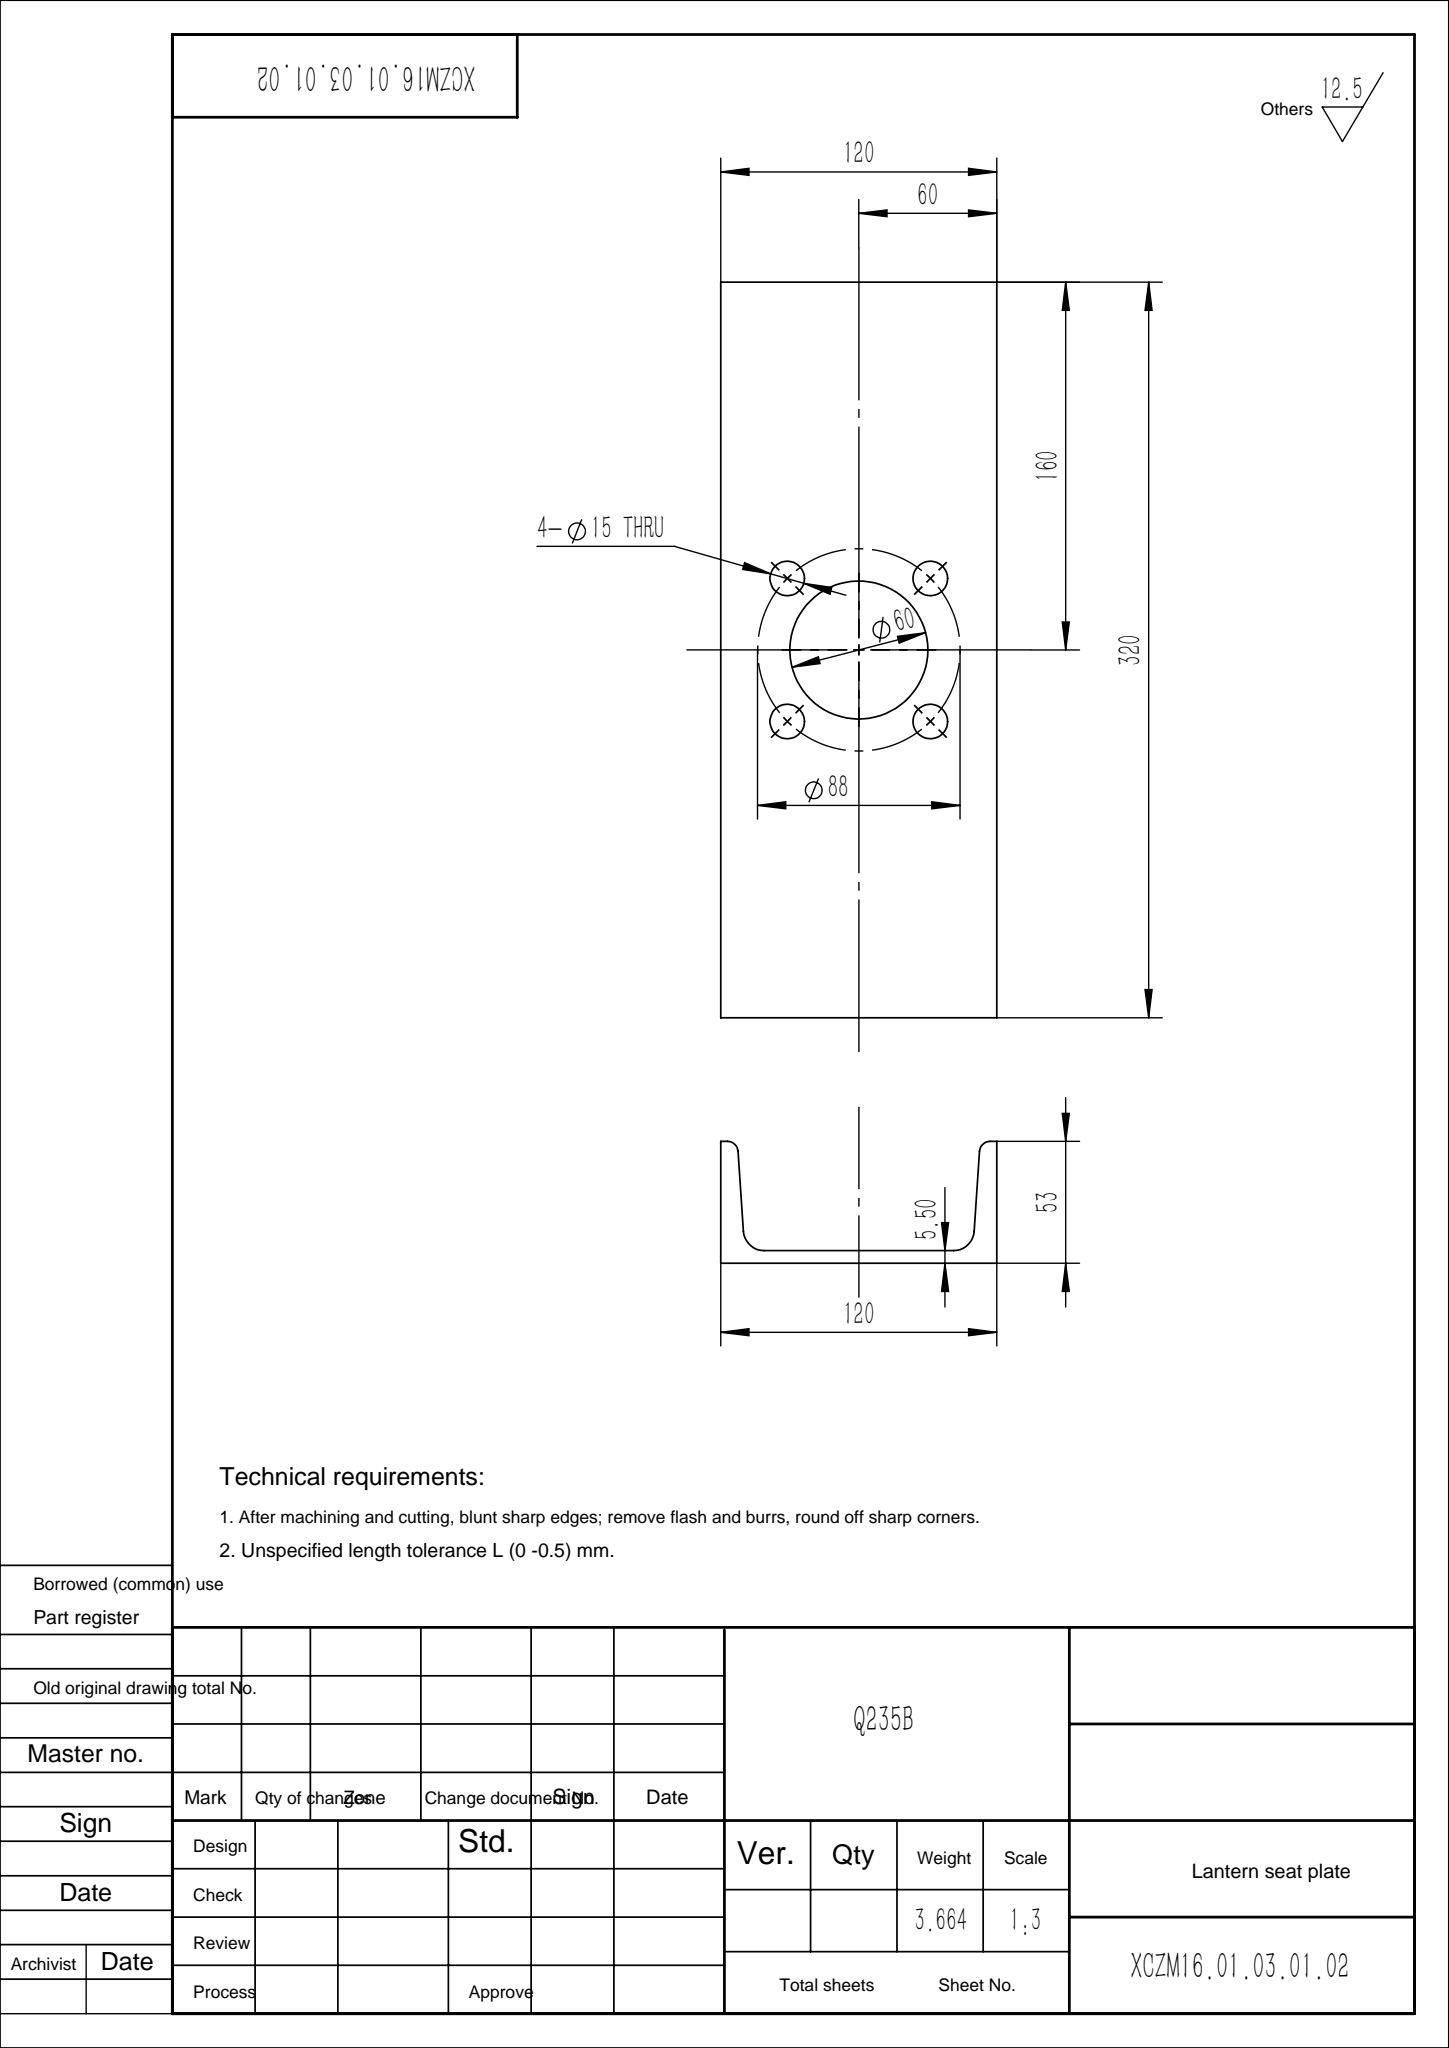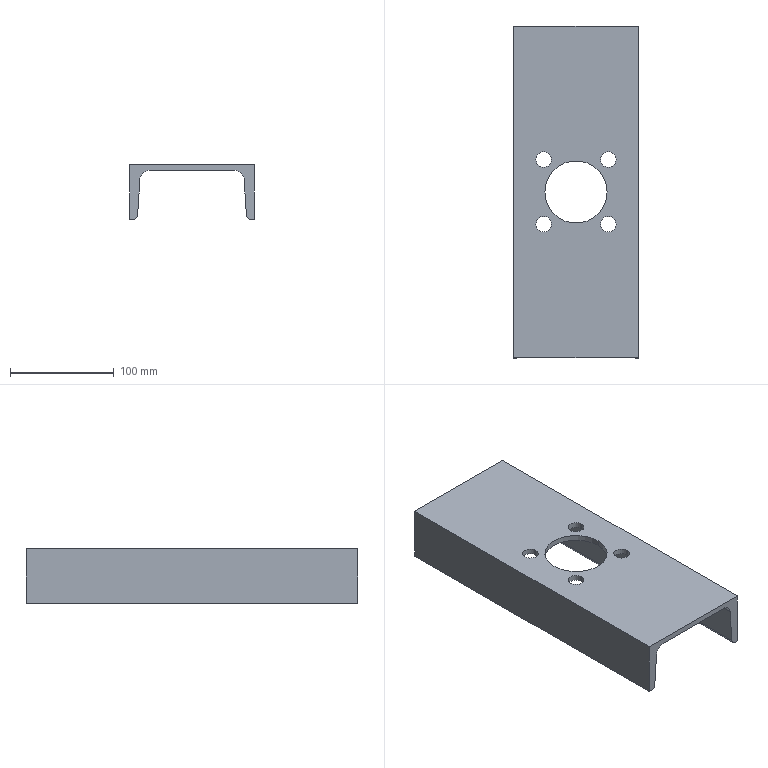Part | SolidWorks | features ICE 1, WeldMemberFeat 1, WeldmentFeature 1 | 1 solid | 24 faces | box 120 x 320 x 53 mm | volume 466744 mm3 | cylinder 14 | plane 10 | commonest cylinder face diameters 15 x8 9 x2 18 x2 60 x2
STEP:
#1=CARTESIAN_POINT('',(-98.613,128.887,-5.5));
#2=VERTEX_POINT('',#1);
#3=CARTESIAN_POINT('',(-83.613,128.887,-5.5));
#4=VERTEX_POINT('',#3);
#5=CARTESIAN_POINT('',(-91.113,128.887,-5.5));
#6=DIRECTION('',(0.,0.,1.));
#7=DIRECTION('',(1.,0.,0.));
#8=AXIS2_PLACEMENT_3D('',#5,#6,#7);
#9=CIRCLE('',#8,7.5);
#10=EDGE_CURVE('',#2,#4,#9,.T.);
#11=ORIENTED_EDGE('',*,*,#10,.F.);
#12=CARTESIAN_POINT('',(-98.613,128.887,0.));
#13=VERTEX_POINT('',#12);
#14=CARTESIAN_POINT('',(-98.613,128.887,-10.));
#15=DIRECTION('',(0.,0.,1.));
#16=VECTOR('',#15,1000.);
#17=LINE('',#14,#16);
#18=EDGE_CURVE('',#2,#13,#17,.T.);
#19=ORIENTED_EDGE('',*,*,#18,.T.);
#20=CARTESIAN_POINT('',(-83.613,128.887,0.));
#21=VERTEX_POINT('',#20);
#22=CARTESIAN_POINT('',(-91.113,128.887,0.));
#23=DIRECTION('',(0.,0.,1.));
#24=DIRECTION('',(1.,0.,0.));
#25=AXIS2_PLACEMENT_3D('',#22,#23,#24);
#26=CIRCLE('',#25,7.5);
#27=EDGE_CURVE('',#13,#21,#26,.T.);
#28=ORIENTED_EDGE('',*,*,#27,.T.);
#29=CARTESIAN_POINT('',(-83.613,128.887,-10.));
#30=DIRECTION('',(0.,0.,1.));
#31=VECTOR('',#30,1000.);
#32=LINE('',#29,#31);
#33=EDGE_CURVE('',#4,#21,#32,.T.);
#34=ORIENTED_EDGE('',*,*,#33,.F.);
#35=EDGE_LOOP('',(#11,#19,#28,#34));
#36=FACE_OUTER_BOUND('',#35,.T.);
#37=CARTESIAN_POINT('',(-91.113,128.887,-10.));
#38=DIRECTION('',(0.,0.,1.));
#39=DIRECTION('',(1.,0.,0.));
#40=AXIS2_PLACEMENT_3D('',#37,#38,#39);
#41=CYLINDRICAL_SURFACE('',#40,7.5);
#42=ADVANCED_FACE('',(#36),#41,.F.);
#43=CARTESIAN_POINT('',(-36.387,128.887,-5.5));
#44=VERTEX_POINT('',#43);
#45=CARTESIAN_POINT('',(-21.387,128.887,-5.5));
#46=VERTEX_POINT('',#45);
#47=CARTESIAN_POINT('',(-28.887,128.887,-5.5));
#48=DIRECTION('',(0.,0.,1.));
#49=DIRECTION('',(1.,0.,0.));
#50=AXIS2_PLACEMENT_3D('',#47,#48,#49);
#51=CIRCLE('',#50,7.5);
#52=EDGE_CURVE('',#44,#46,#51,.T.);
#53=ORIENTED_EDGE('',*,*,#52,.F.);
#54=CARTESIAN_POINT('',(-36.387,128.887,0.));
#55=VERTEX_POINT('',#54);
#56=CARTESIAN_POINT('',(-36.387,128.887,-10.));
#57=DIRECTION('',(0.,0.,1.));
#58=VECTOR('',#57,1000.);
#59=LINE('',#56,#58);
#60=EDGE_CURVE('',#44,#55,#59,.T.);
#61=ORIENTED_EDGE('',*,*,#60,.T.);
#62=CARTESIAN_POINT('',(-21.387,128.887,0.));
#63=VERTEX_POINT('',#62);
#64=CARTESIAN_POINT('',(-28.887,128.887,0.));
#65=DIRECTION('',(0.,0.,1.));
#66=DIRECTION('',(1.,0.,0.));
#67=AXIS2_PLACEMENT_3D('',#64,#65,#66);
#68=CIRCLE('',#67,7.5);
#69=EDGE_CURVE('',#55,#63,#68,.T.);
#70=ORIENTED_EDGE('',*,*,#69,.T.);
#71=CARTESIAN_POINT('',(-21.387,128.887,-10.));
#72=DIRECTION('',(0.,0.,1.));
#73=VECTOR('',#72,1000.);
#74=LINE('',#71,#73);
#75=EDGE_CURVE('',#46,#63,#74,.T.);
#76=ORIENTED_EDGE('',*,*,#75,.F.);
#77=EDGE_LOOP('',(#53,#61,#70,#76));
#78=FACE_OUTER_BOUND('',#77,.T.);
#79=CARTESIAN_POINT('',(-28.887,128.887,-10.));
#80=DIRECTION('',(0.,0.,1.));
#81=DIRECTION('',(1.,0.,0.));
#82=AXIS2_PLACEMENT_3D('',#79,#80,#81);
#83=CYLINDRICAL_SURFACE('',#82,7.5);
#84=ADVANCED_FACE('',(#78),#83,.F.);
#85=CARTESIAN_POINT('',(-36.387,191.113,-5.5));
#86=VERTEX_POINT('',#85);
#87=CARTESIAN_POINT('',(-21.387,191.113,-5.5));
#88=VERTEX_POINT('',#87);
#89=CARTESIAN_POINT('',(-28.887,191.113,-5.5));
#90=DIRECTION('',(0.,0.,1.));
#91=DIRECTION('',(1.,0.,0.));
#92=AXIS2_PLACEMENT_3D('',#89,#90,#91);
#93=CIRCLE('',#92,7.5);
#94=EDGE_CURVE('',#86,#88,#93,.T.);
#95=ORIENTED_EDGE('',*,*,#94,.F.);
#96=CARTESIAN_POINT('',(-36.387,191.113,0.));
#97=VERTEX_POINT('',#96);
#98=CARTESIAN_POINT('',(-36.387,191.113,-10.));
#99=DIRECTION('',(0.,0.,1.));
#100=VECTOR('',#99,1000.);
#101=LINE('',#98,#100);
#102=EDGE_CURVE('',#86,#97,#101,.T.);
#103=ORIENTED_EDGE('',*,*,#102,.T.);
#104=CARTESIAN_POINT('',(-21.387,191.113,0.));
#105=VERTEX_POINT('',#104);
#106=CARTESIAN_POINT('',(-28.887,191.113,0.));
#107=DIRECTION('',(0.,0.,1.));
#108=DIRECTION('',(1.,0.,0.));
#109=AXIS2_PLACEMENT_3D('',#106,#107,#108);
#110=CIRCLE('',#109,7.5);
#111=EDGE_CURVE('',#97,#105,#110,.T.);
#112=ORIENTED_EDGE('',*,*,#111,.T.);
#113=CARTESIAN_POINT('',(-21.387,191.113,-10.));
#114=DIRECTION('',(0.,0.,1.));
#115=VECTOR('',#114,1000.);
#116=LINE('',#113,#115);
#117=EDGE_CURVE('',#88,#105,#116,.T.);
#118=ORIENTED_EDGE('',*,*,#117,.F.);
#119=EDGE_LOOP('',(#95,#103,#112,#118));
#120=FACE_OUTER_BOUND('',#119,.T.);
#121=CARTESIAN_POINT('',(-28.887,191.113,-10.));
#122=DIRECTION('',(0.,0.,1.));
#123=DIRECTION('',(1.,0.,0.));
#124=AXIS2_PLACEMENT_3D('',#121,#122,#123);
#125=CYLINDRICAL_SURFACE('',#124,7.5);
#126=ADVANCED_FACE('',(#120),#125,.F.);
#127=CARTESIAN_POINT('',(-98.613,191.113,-5.5));
#128=VERTEX_POINT('',#127);
#129=CARTESIAN_POINT('',(-83.613,191.113,-5.5));
#130=VERTEX_POINT('',#129);
#131=CARTESIAN_POINT('',(-91.113,191.113,-5.5));
#132=DIRECTION('',(0.,0.,1.));
#133=DIRECTION('',(1.,0.,0.));
#134=AXIS2_PLACEMENT_3D('',#131,#132,#133);
#135=CIRCLE('',#134,7.5);
#136=EDGE_CURVE('',#128,#130,#135,.T.);
#137=ORIENTED_EDGE('',*,*,#136,.F.);
#138=CARTESIAN_POINT('',(-98.613,191.113,0.));
#139=VERTEX_POINT('',#138);
#140=CARTESIAN_POINT('',(-98.613,191.113,-10.));
#141=DIRECTION('',(0.,0.,1.));
#142=VECTOR('',#141,1000.);
#143=LINE('',#140,#142);
#144=EDGE_CURVE('',#128,#139,#143,.T.);
#145=ORIENTED_EDGE('',*,*,#144,.T.);
#146=CARTESIAN_POINT('',(-83.613,191.113,0.));
#147=VERTEX_POINT('',#146);
#148=CARTESIAN_POINT('',(-91.113,191.113,0.));
#149=DIRECTION('',(0.,0.,1.));
#150=DIRECTION('',(1.,0.,0.));
#151=AXIS2_PLACEMENT_3D('',#148,#149,#150);
#152=CIRCLE('',#151,7.5);
#153=EDGE_CURVE('',#139,#147,#152,.T.);
#154=ORIENTED_EDGE('',*,*,#153,.T.);
#155=CARTESIAN_POINT('',(-83.613,191.113,-10.));
#156=DIRECTION('',(0.,0.,1.));
#157=VECTOR('',#156,1000.);
#158=LINE('',#155,#157);
#159=EDGE_CURVE('',#130,#147,#158,.T.);
#160=ORIENTED_EDGE('',*,*,#159,.F.);
#161=EDGE_LOOP('',(#137,#145,#154,#160));
#162=FACE_OUTER_BOUND('',#161,.T.);
#163=CARTESIAN_POINT('',(-91.113,191.113,-10.));
#164=DIRECTION('',(0.,0.,1.));
#165=DIRECTION('',(1.,0.,0.));
#166=AXIS2_PLACEMENT_3D('',#163,#164,#165);
#167=CYLINDRICAL_SURFACE('',#166,7.5);
#168=ADVANCED_FACE('',(#162),#167,.F.);
#169=CARTESIAN_POINT('',(-90.,160.,-5.5));
#170=VERTEX_POINT('',#169);
#171=CARTESIAN_POINT('',(-30.,160.,-5.5));
#172=VERTEX_POINT('',#171);
#173=CARTESIAN_POINT('',(-60.,160.,-5.5));
#174=DIRECTION('',(0.,0.,1.));
#175=DIRECTION('',(1.,0.,0.));
#176=AXIS2_PLACEMENT_3D('',#173,#174,#175);
#177=CIRCLE('',#176,30.);
#178=EDGE_CURVE('',#170,#172,#177,.T.);
#179=ORIENTED_EDGE('',*,*,#178,.F.);
#180=CARTESIAN_POINT('',(-90.,160.,0.));
#181=VERTEX_POINT('',#180);
#182=CARTESIAN_POINT('',(-90.,160.,-10.));
#183=DIRECTION('',(0.,0.,1.));
#184=VECTOR('',#183,1000.);
#185=LINE('',#182,#184);
#186=EDGE_CURVE('',#170,#181,#185,.T.);
#187=ORIENTED_EDGE('',*,*,#186,.T.);
#188=CARTESIAN_POINT('',(-30.,160.,0.));
#189=VERTEX_POINT('',#188);
#190=CARTESIAN_POINT('',(-60.,160.,0.));
#191=DIRECTION('',(0.,0.,1.));
#192=DIRECTION('',(1.,0.,0.));
#193=AXIS2_PLACEMENT_3D('',#190,#191,#192);
#194=CIRCLE('',#193,30.);
#195=EDGE_CURVE('',#181,#189,#194,.T.);
#196=ORIENTED_EDGE('',*,*,#195,.T.);
#197=CARTESIAN_POINT('',(-30.,160.,-10.));
#198=DIRECTION('',(0.,0.,1.));
#199=VECTOR('',#198,1000.);
#200=LINE('',#197,#199);
#201=EDGE_CURVE('',#172,#189,#200,.T.);
#202=ORIENTED_EDGE('',*,*,#201,.F.);
#203=EDGE_LOOP('',(#179,#187,#196,#202));
#204=FACE_OUTER_BOUND('',#203,.T.);
#205=CARTESIAN_POINT('',(-60.,160.,-10.));
#206=DIRECTION('',(0.,0.,1.));
#207=DIRECTION('',(1.,0.,0.));
#208=AXIS2_PLACEMENT_3D('',#205,#206,#207);
#209=CYLINDRICAL_SURFACE('',#208,30.);
#210=ADVANCED_FACE('',(#204),#209,.F.);
#211=CARTESIAN_POINT('',(-120.,0.,-53.));
#212=VERTEX_POINT('',#211);
#213=CARTESIAN_POINT('',(-120.,0.,0.));
#214=VERTEX_POINT('',#213);
#215=CARTESIAN_POINT('',(-120.,0.,0.));
#216=DIRECTION('',(0.,0.,1.));
#217=VECTOR('',#216,1000.);
#218=LINE('',#215,#217);
#219=EDGE_CURVE('',#212,#214,#218,.T.);
#220=ORIENTED_EDGE('',*,*,#219,.T.);
#221=CARTESIAN_POINT('',(-120.,320.,0.));
#222=VERTEX_POINT('',#221);
#223=CARTESIAN_POINT('',(-120.,320.,0.));
#224=DIRECTION('',(0.,-1.,0.));
#225=VECTOR('',#224,1000.);
#226=LINE('',#223,#225);
#227=EDGE_CURVE('',#222,#214,#226,.T.);
#228=ORIENTED_EDGE('',*,*,#227,.F.);
#229=CARTESIAN_POINT('',(-120.,320.,-53.));
#230=VERTEX_POINT('',#229);
#231=CARTESIAN_POINT('',(-120.,320.,0.));
#232=DIRECTION('',(0.,0.,1.));
#233=VECTOR('',#232,1000.);
#234=LINE('',#231,#233);
#235=EDGE_CURVE('',#230,#222,#234,.T.);
#236=ORIENTED_EDGE('',*,*,#235,.F.);
#237=CARTESIAN_POINT('',(-120.,320.,-53.));
#238=DIRECTION('',(0.,-1.,0.));
#239=VECTOR('',#238,1000.);
#240=LINE('',#237,#239);
#241=EDGE_CURVE('',#230,#212,#240,.T.);
#242=ORIENTED_EDGE('',*,*,#241,.T.);
#243=EDGE_LOOP('',(#220,#228,#236,#242));
#244=FACE_OUTER_BOUND('',#243,.T.);
#245=CARTESIAN_POINT('',(-120.,320.,0.));
#246=DIRECTION('',(1.,0.,0.));
#247=DIRECTION('',(0.,0.,-1.));
#248=AXIS2_PLACEMENT_3D('',#245,#246,#247);
#249=PLANE('',#248);
#250=ADVANCED_FACE('',(#244),#249,.F.);
#251=CARTESIAN_POINT('',(-91.113,128.887,0.));
#252=DIRECTION('',(0.,0.,1.));
#253=DIRECTION('',(1.,0.,0.));
#254=AXIS2_PLACEMENT_3D('',#251,#252,#253);
#255=CIRCLE('',#254,7.5);
#256=EDGE_CURVE('',#21,#13,#255,.T.);
#257=ORIENTED_EDGE('',*,*,#256,.F.);
#258=ORIENTED_EDGE('',*,*,#27,.F.);
#259=EDGE_LOOP('',(#257,#258));
#260=FACE_BOUND('',#259,.T.);
#261=CARTESIAN_POINT('',(-28.887,128.887,0.));
#262=DIRECTION('',(0.,0.,1.));
#263=DIRECTION('',(1.,0.,0.));
#264=AXIS2_PLACEMENT_3D('',#261,#262,#263);
#265=CIRCLE('',#264,7.5);
#266=EDGE_CURVE('',#63,#55,#265,.T.);
#267=ORIENTED_EDGE('',*,*,#266,.F.);
#268=ORIENTED_EDGE('',*,*,#69,.F.);
#269=EDGE_LOOP('',(#267,#268));
#270=FACE_BOUND('',#269,.T.);
#271=CARTESIAN_POINT('',(-28.887,191.113,0.));
#272=DIRECTION('',(0.,0.,1.));
#273=DIRECTION('',(1.,0.,0.));
#274=AXIS2_PLACEMENT_3D('',#271,#272,#273);
#275=CIRCLE('',#274,7.5);
#276=EDGE_CURVE('',#105,#97,#275,.T.);
#277=ORIENTED_EDGE('',*,*,#276,.F.);
#278=ORIENTED_EDGE('',*,*,#111,.F.);
#279=EDGE_LOOP('',(#277,#278));
#280=FACE_BOUND('',#279,.T.);
#281=CARTESIAN_POINT('',(-91.113,191.113,0.));
#282=DIRECTION('',(0.,0.,1.));
#283=DIRECTION('',(1.,0.,0.));
#284=AXIS2_PLACEMENT_3D('',#281,#282,#283);
#285=CIRCLE('',#284,7.5);
#286=EDGE_CURVE('',#147,#139,#285,.T.);
#287=ORIENTED_EDGE('',*,*,#286,.F.);
#288=ORIENTED_EDGE('',*,*,#153,.F.);
#289=EDGE_LOOP('',(#287,#288));
#290=FACE_BOUND('',#289,.T.);
#291=CARTESIAN_POINT('',(-60.,160.,0.));
#292=DIRECTION('',(0.,0.,1.));
#293=DIRECTION('',(1.,0.,0.));
#294=AXIS2_PLACEMENT_3D('',#291,#292,#293);
#295=CIRCLE('',#294,30.);
#296=EDGE_CURVE('',#189,#181,#295,.T.);
#297=ORIENTED_EDGE('',*,*,#296,.F.);
#298=ORIENTED_EDGE('',*,*,#195,.F.);
#299=EDGE_LOOP('',(#297,#298));
#300=FACE_BOUND('',#299,.T.);
#301=CARTESIAN_POINT('',(0.,0.,0.));
#302=VERTEX_POINT('',#301);
#303=CARTESIAN_POINT('',(0.,0.,0.));
#304=DIRECTION('',(1.,0.,0.));
#305=VECTOR('',#304,1000.);
#306=LINE('',#303,#305);
#307=EDGE_CURVE('',#214,#302,#306,.T.);
#308=ORIENTED_EDGE('',*,*,#307,.T.);
#309=CARTESIAN_POINT('',(0.,320.,0.));
#310=VERTEX_POINT('',#309);
#311=CARTESIAN_POINT('',(0.,320.,0.));
#312=DIRECTION('',(0.,-1.,0.));
#313=VECTOR('',#312,1000.);
#314=LINE('',#311,#313);
#315=EDGE_CURVE('',#310,#302,#314,.T.);
#316=ORIENTED_EDGE('',*,*,#315,.F.);
#317=CARTESIAN_POINT('',(0.,320.,0.));
#318=DIRECTION('',(1.,0.,0.));
#319=VECTOR('',#318,1000.);
#320=LINE('',#317,#319);
#321=EDGE_CURVE('',#222,#310,#320,.T.);
#322=ORIENTED_EDGE('',*,*,#321,.F.);
#323=ORIENTED_EDGE('',*,*,#227,.T.);
#324=EDGE_LOOP('',(#308,#316,#322,#323));
#325=FACE_OUTER_BOUND('',#324,.T.);
#326=CARTESIAN_POINT('',(0.,320.,0.));
#327=DIRECTION('',(0.,0.,-1.));
#328=DIRECTION('',(-1.,0.,0.));
#329=AXIS2_PLACEMENT_3D('',#326,#327,#328);
#330=PLANE('',#329);
#331=ADVANCED_FACE('',(#260,#270,#280,#290,#300,#325),#330,.F.);
#332=CARTESIAN_POINT('',(0.,0.,-53.));
#333=VERTEX_POINT('',#332);
#334=CARTESIAN_POINT('',(0.,0.,0.));
#335=DIRECTION('',(0.,0.,-1.));
#336=VECTOR('',#335,1000.);
#337=LINE('',#334,#336);
#338=EDGE_CURVE('',#302,#333,#337,.T.);
#339=ORIENTED_EDGE('',*,*,#338,.T.);
#340=CARTESIAN_POINT('',(0.,320.,-53.));
#341=VERTEX_POINT('',#340);
#342=CARTESIAN_POINT('',(0.,320.,-53.));
#343=DIRECTION('',(0.,-1.,0.));
#344=VECTOR('',#343,1000.);
#345=LINE('',#342,#344);
#346=EDGE_CURVE('',#341,#333,#345,.T.);
#347=ORIENTED_EDGE('',*,*,#346,.F.);
#348=CARTESIAN_POINT('',(0.,320.,0.));
#349=DIRECTION('',(0.,0.,-1.));
#350=VECTOR('',#349,1000.);
#351=LINE('',#348,#350);
#352=EDGE_CURVE('',#310,#341,#351,.T.);
#353=ORIENTED_EDGE('',*,*,#352,.F.);
#354=ORIENTED_EDGE('',*,*,#315,.T.);
#355=EDGE_LOOP('',(#339,#347,#353,#354));
#356=FACE_OUTER_BOUND('',#355,.T.);
#357=CARTESIAN_POINT('',(0.,320.,0.));
#358=DIRECTION('',(-1.,0.,0.));
#359=DIRECTION('',(0.,0.,1.));
#360=AXIS2_PLACEMENT_3D('',#357,#358,#359);
#361=PLANE('',#360);
#362=ADVANCED_FACE('',(#356),#361,.F.);
#363=CARTESIAN_POINT('',(-2.984,0.,-53.));
#364=VERTEX_POINT('',#363);
#365=CARTESIAN_POINT('',(-2.984,0.,-53.));
#366=DIRECTION('',(-1.,0.,0.));
#367=VECTOR('',#366,1000.);
#368=LINE('',#365,#367);
#369=EDGE_CURVE('',#333,#364,#368,.T.);
#370=ORIENTED_EDGE('',*,*,#369,.T.);
#371=CARTESIAN_POINT('',(-2.984,320.,-53.));
#372=VERTEX_POINT('',#371);
#373=CARTESIAN_POINT('',(-2.984,320.,-53.));
#374=DIRECTION('',(0.,-1.,0.));
#375=VECTOR('',#374,1000.);
#376=LINE('',#373,#375);
#377=EDGE_CURVE('',#372,#364,#376,.T.);
#378=ORIENTED_EDGE('',*,*,#377,.F.);
#379=CARTESIAN_POINT('',(-2.984,320.,-53.));
#380=DIRECTION('',(-1.,0.,0.));
#381=VECTOR('',#380,1000.);
#382=LINE('',#379,#381);
#383=EDGE_CURVE('',#341,#372,#382,.T.);
#384=ORIENTED_EDGE('',*,*,#383,.F.);
#385=ORIENTED_EDGE('',*,*,#346,.T.);
#386=EDGE_LOOP('',(#370,#378,#384,#385));
#387=FACE_OUTER_BOUND('',#386,.T.);
#388=CARTESIAN_POINT('',(-2.984,320.,-53.));
#389=DIRECTION('',(0.,0.,1.));
#390=DIRECTION('',(1.,0.,0.));
#391=AXIS2_PLACEMENT_3D('',#388,#389,#390);
#392=PLANE('',#391);
#393=ADVANCED_FACE('',(#387),#392,.F.);
#394=CARTESIAN_POINT('',(-7.474,0.,-48.807));
#395=VERTEX_POINT('',#394);
#396=CARTESIAN_POINT('',(-2.984,0.,-48.5));
#397=DIRECTION('',(0.,1.,0.));
#398=DIRECTION('',(0.,0.,1.));
#399=AXIS2_PLACEMENT_3D('',#396,#397,#398);
#400=CIRCLE('',#399,4.5);
#401=EDGE_CURVE('',#364,#395,#400,.T.);
#402=ORIENTED_EDGE('',*,*,#401,.T.);
#403=CARTESIAN_POINT('',(-7.474,320.,-48.807));
#404=VERTEX_POINT('',#403);
#405=CARTESIAN_POINT('',(-7.474,320.,-48.807));
#406=DIRECTION('',(0.,-1.,0.));
#407=VECTOR('',#406,1000.);
#408=LINE('',#405,#407);
#409=EDGE_CURVE('',#404,#395,#408,.T.);
#410=ORIENTED_EDGE('',*,*,#409,.F.);
#411=CARTESIAN_POINT('',(-2.984,320.,-48.5));
#412=DIRECTION('',(0.,1.,0.));
#413=DIRECTION('',(0.,0.,1.));
#414=AXIS2_PLACEMENT_3D('',#411,#412,#413);
#415=CIRCLE('',#414,4.5);
#416=EDGE_CURVE('',#372,#404,#415,.T.);
#417=ORIENTED_EDGE('',*,*,#416,.F.);
#418=ORIENTED_EDGE('',*,*,#377,.T.);
#419=EDGE_LOOP('',(#402,#410,#417,#418));
#420=FACE_OUTER_BOUND('',#419,.T.);
#421=CARTESIAN_POINT('',(-2.984,320.,-48.5));
#422=DIRECTION('',(0.,-1.,0.));
#423=DIRECTION('',(0.,0.,-1.));
#424=AXIS2_PLACEMENT_3D('',#421,#422,#423);
#425=CYLINDRICAL_SURFACE('',#424,4.5);
#426=ADVANCED_FACE('',(#420),#425,.T.);
#427=CARTESIAN_POINT('',(-9.863,0.,-13.886));
#428=VERTEX_POINT('',#427);
#429=CARTESIAN_POINT('',(-9.863,0.,-13.886));
#430=DIRECTION('',(-0.06826,0.,0.9977));
#431=VECTOR('',#430,1000.);
#432=LINE('',#429,#431);
#433=EDGE_CURVE('',#395,#428,#432,.T.);
#434=ORIENTED_EDGE('',*,*,#433,.T.);
#435=CARTESIAN_POINT('',(-9.863,320.,-13.886));
#436=VERTEX_POINT('',#435);
#437=CARTESIAN_POINT('',(-9.863,320.,-13.886));
#438=DIRECTION('',(0.,-1.,0.));
#439=VECTOR('',#438,1000.);
#440=LINE('',#437,#439);
#441=EDGE_CURVE('',#436,#428,#440,.T.);
#442=ORIENTED_EDGE('',*,*,#441,.F.);
#443=CARTESIAN_POINT('',(-9.863,320.,-13.886));
#444=DIRECTION('',(-0.06826,0.,0.9977));
#445=VECTOR('',#444,1000.);
#446=LINE('',#443,#445);
#447=EDGE_CURVE('',#404,#436,#446,.T.);
#448=ORIENTED_EDGE('',*,*,#447,.F.);
#449=ORIENTED_EDGE('',*,*,#409,.T.);
#450=EDGE_LOOP('',(#434,#442,#448,#449));
#451=FACE_OUTER_BOUND('',#450,.T.);
#452=CARTESIAN_POINT('',(-9.863,320.,-13.886));
#453=DIRECTION('',(0.9977,0.,0.06826));
#454=DIRECTION('',(0.06826,0.,-0.9977));
#455=AXIS2_PLACEMENT_3D('',#452,#453,#454);
#456=PLANE('',#455);
#457=ADVANCED_FACE('',(#451),#456,.F.);
#458=CARTESIAN_POINT('',(-18.842,0.,-5.5));
#459=VERTEX_POINT('',#458);
#460=CARTESIAN_POINT('',(-18.842,0.,-14.5));
#461=DIRECTION('',(0.,-1.,0.));
#462=DIRECTION('',(0.,0.,-1.));
#463=AXIS2_PLACEMENT_3D('',#460,#461,#462);
#464=CIRCLE('',#463,9.);
#465=EDGE_CURVE('',#428,#459,#464,.T.);
#466=ORIENTED_EDGE('',*,*,#465,.T.);
#467=CARTESIAN_POINT('',(-18.842,320.,-5.5));
#468=VERTEX_POINT('',#467);
#469=CARTESIAN_POINT('',(-18.842,320.,-5.5));
#470=DIRECTION('',(0.,-1.,0.));
#471=VECTOR('',#470,1000.);
#472=LINE('',#469,#471);
#473=EDGE_CURVE('',#468,#459,#472,.T.);
#474=ORIENTED_EDGE('',*,*,#473,.F.);
#475=CARTESIAN_POINT('',(-18.842,320.,-14.5));
#476=DIRECTION('',(0.,-1.,0.));
#477=DIRECTION('',(0.,0.,-1.));
#478=AXIS2_PLACEMENT_3D('',#475,#476,#477);
#479=CIRCLE('',#478,9.);
#480=EDGE_CURVE('',#436,#468,#479,.T.);
#481=ORIENTED_EDGE('',*,*,#480,.F.);
#482=ORIENTED_EDGE('',*,*,#441,.T.);
#483=EDGE_LOOP('',(#466,#474,#481,#482));
#484=FACE_OUTER_BOUND('',#483,.T.);
#485=CARTESIAN_POINT('',(-18.842,320.,-14.5));
#486=DIRECTION('',(0.,-1.,0.));
#487=DIRECTION('',(0.,0.,-1.));
#488=AXIS2_PLACEMENT_3D('',#485,#486,#487);
#489=CYLINDRICAL_SURFACE('',#488,9.);
#490=ADVANCED_FACE('',(#484),#489,.F.);
#491=CARTESIAN_POINT('',(-91.113,128.887,-5.5));
#492=DIRECTION('',(0.,0.,1.));
#493=DIRECTION('',(1.,0.,0.));
#494=AXIS2_PLACEMENT_3D('',#491,#492,#493);
#495=CIRCLE('',#494,7.5);
#496=EDGE_CURVE('',#4,#2,#495,.T.);
#497=ORIENTED_EDGE('',*,*,#496,.T.);
#498=ORIENTED_EDGE('',*,*,#10,.T.);
#499=EDGE_LOOP('',(#497,#498));
#500=FACE_BOUND('',#499,.T.);
#501=CARTESIAN_POINT('',(-28.887,128.887,-5.5));
#502=DIRECTION('',(0.,0.,1.));
#503=DIRECTION('',(1.,0.,0.));
#504=AXIS2_PLACEMENT_3D('',#501,#502,#503);
#505=CIRCLE('',#504,7.5);
#506=EDGE_CURVE('',#46,#44,#505,.T.);
#507=ORIENTED_EDGE('',*,*,#506,.T.);
#508=ORIENTED_EDGE('',*,*,#52,.T.);
#509=EDGE_LOOP('',(#507,#508));
#510=FACE_BOUND('',#509,.T.);
#511=CARTESIAN_POINT('',(-28.887,191.113,-5.5));
#512=DIRECTION('',(0.,0.,1.));
#513=DIRECTION('',(1.,0.,0.));
#514=AXIS2_PLACEMENT_3D('',#511,#512,#513);
#515=CIRCLE('',#514,7.5);
#516=EDGE_CURVE('',#88,#86,#515,.T.);
#517=ORIENTED_EDGE('',*,*,#516,.T.);
#518=ORIENTED_EDGE('',*,*,#94,.T.);
#519=EDGE_LOOP('',(#517,#518));
#520=FACE_BOUND('',#519,.T.);
#521=CARTESIAN_POINT('',(-91.113,191.113,-5.5));
#522=DIRECTION('',(0.,0.,1.));
#523=DIRECTION('',(1.,0.,0.));
#524=AXIS2_PLACEMENT_3D('',#521,#522,#523);
#525=CIRCLE('',#524,7.5);
#526=EDGE_CURVE('',#130,#128,#525,.T.);
#527=ORIENTED_EDGE('',*,*,#526,.T.);
#528=ORIENTED_EDGE('',*,*,#136,.T.);
#529=EDGE_LOOP('',(#527,#528));
#530=FACE_BOUND('',#529,.T.);
#531=CARTESIAN_POINT('',(-60.,160.,-5.5));
#532=DIRECTION('',(0.,0.,1.));
#533=DIRECTION('',(1.,0.,0.));
#534=AXIS2_PLACEMENT_3D('',#531,#532,#533);
#535=CIRCLE('',#534,30.);
#536=EDGE_CURVE('',#172,#170,#535,.T.);
#537=ORIENTED_EDGE('',*,*,#536,.T.);
#538=ORIENTED_EDGE('',*,*,#178,.T.);
#539=EDGE_LOOP('',(#537,#538));
#540=FACE_BOUND('',#539,.T.);
#541=CARTESIAN_POINT('',(-101.158,0.,-5.5));
#542=VERTEX_POINT('',#541);
#543=CARTESIAN_POINT('',(-101.158,0.,-5.5));
#544=DIRECTION('',(-1.,0.,0.));
#545=VECTOR('',#544,1000.);
#546=LINE('',#543,#545);
#547=EDGE_CURVE('',#459,#542,#546,.T.);
#548=ORIENTED_EDGE('',*,*,#547,.T.);
#549=CARTESIAN_POINT('',(-101.158,320.,-5.5));
#550=VERTEX_POINT('',#549);
#551=CARTESIAN_POINT('',(-101.158,320.,-5.5));
#552=DIRECTION('',(0.,-1.,0.));
#553=VECTOR('',#552,1000.);
#554=LINE('',#551,#553);
#555=EDGE_CURVE('',#550,#542,#554,.T.);
#556=ORIENTED_EDGE('',*,*,#555,.F.);
#557=CARTESIAN_POINT('',(-101.158,320.,-5.5));
#558=DIRECTION('',(-1.,0.,0.));
#559=VECTOR('',#558,1000.);
#560=LINE('',#557,#559);
#561=EDGE_CURVE('',#468,#550,#560,.T.);
#562=ORIENTED_EDGE('',*,*,#561,.F.);
#563=ORIENTED_EDGE('',*,*,#473,.T.);
#564=EDGE_LOOP('',(#548,#556,#562,#563));
#565=FACE_OUTER_BOUND('',#564,.T.);
#566=CARTESIAN_POINT('',(-101.158,320.,-5.5));
#567=DIRECTION('',(0.,0.,1.));
#568=DIRECTION('',(1.,0.,0.));
#569=AXIS2_PLACEMENT_3D('',#566,#567,#568);
#570=PLANE('',#569);
#571=ADVANCED_FACE('',(#500,#510,#520,#530,#540,#565),#570,.F.);
#572=CARTESIAN_POINT('',(-110.137,0.,-13.886));
#573=VERTEX_POINT('',#572);
#574=CARTESIAN_POINT('',(-101.158,0.,-14.5));
#575=DIRECTION('',(0.,-1.,0.));
#576=DIRECTION('',(0.,0.,-1.));
#577=AXIS2_PLACEMENT_3D('',#574,#575,#576);
#578=CIRCLE('',#577,9.);
#579=EDGE_CURVE('',#542,#573,#578,.T.);
#580=ORIENTED_EDGE('',*,*,#579,.T.);
#581=CARTESIAN_POINT('',(-110.137,320.,-13.886));
#582=VERTEX_POINT('',#581);
#583=CARTESIAN_POINT('',(-110.137,320.,-13.886));
#584=DIRECTION('',(0.,-1.,0.));
#585=VECTOR('',#584,1000.);
#586=LINE('',#583,#585);
#587=EDGE_CURVE('',#582,#573,#586,.T.);
#588=ORIENTED_EDGE('',*,*,#587,.F.);
#589=CARTESIAN_POINT('',(-101.158,320.,-14.5));
#590=DIRECTION('',(0.,-1.,0.));
#591=DIRECTION('',(0.,0.,-1.));
#592=AXIS2_PLACEMENT_3D('',#589,#590,#591);
#593=CIRCLE('',#592,9.);
#594=EDGE_CURVE('',#550,#582,#593,.T.);
#595=ORIENTED_EDGE('',*,*,#594,.F.);
#596=ORIENTED_EDGE('',*,*,#555,.T.);
#597=EDGE_LOOP('',(#580,#588,#595,#596));
#598=FACE_OUTER_BOUND('',#597,.T.);
#599=CARTESIAN_POINT('',(-101.158,320.,-14.5));
#600=DIRECTION('',(0.,-1.,0.));
#601=DIRECTION('',(0.,0.,-1.));
#602=AXIS2_PLACEMENT_3D('',#599,#600,#601);
#603=CYLINDRICAL_SURFACE('',#602,9.);
#604=ADVANCED_FACE('',(#598),#603,.F.);
#605=CARTESIAN_POINT('',(-112.526,0.,-48.807));
#606=VERTEX_POINT('',#605);
#607=CARTESIAN_POINT('',(-110.137,0.,-13.886));
#608=DIRECTION('',(-0.06826,0.,-0.9977));
#609=VECTOR('',#608,1000.);
#610=LINE('',#607,#609);
#611=EDGE_CURVE('',#573,#606,#610,.T.);
#612=ORIENTED_EDGE('',*,*,#611,.T.);
#613=CARTESIAN_POINT('',(-112.526,320.,-48.807));
#614=VERTEX_POINT('',#613);
#615=CARTESIAN_POINT('',(-112.526,320.,-48.807));
#616=DIRECTION('',(0.,-1.,0.));
#617=VECTOR('',#616,1000.);
#618=LINE('',#615,#617);
#619=EDGE_CURVE('',#614,#606,#618,.T.);
#620=ORIENTED_EDGE('',*,*,#619,.F.);
#621=CARTESIAN_POINT('',(-110.137,320.,-13.886));
#622=DIRECTION('',(-0.06826,0.,-0.9977));
#623=VECTOR('',#622,1000.);
#624=LINE('',#621,#623);
#625=EDGE_CURVE('',#582,#614,#624,.T.);
#626=ORIENTED_EDGE('',*,*,#625,.F.);
#627=ORIENTED_EDGE('',*,*,#587,.T.);
#628=EDGE_LOOP('',(#612,#620,#626,#627));
#629=FACE_OUTER_BOUND('',#628,.T.);
#630=CARTESIAN_POINT('',(-110.137,320.,-13.886));
#631=DIRECTION('',(-0.9977,0.,0.06826));
#632=DIRECTION('',(0.06826,0.,0.9977));
#633=AXIS2_PLACEMENT_3D('',#630,#631,#632);
#634=PLANE('',#633);
#635=ADVANCED_FACE('',(#629),#634,.F.);
#636=CARTESIAN_POINT('',(-117.016,0.,-53.));
#637=VERTEX_POINT('',#636);
#638=CARTESIAN_POINT('',(-117.016,0.,-48.5));
#639=DIRECTION('',(0.,1.,0.));
#640=DIRECTION('',(0.,0.,1.));
#641=AXIS2_PLACEMENT_3D('',#638,#639,#640);
#642=CIRCLE('',#641,4.5);
#643=EDGE_CURVE('',#606,#637,#642,.T.);
#644=ORIENTED_EDGE('',*,*,#643,.T.);
#645=CARTESIAN_POINT('',(-117.016,320.,-53.));
#646=VERTEX_POINT('',#645);
#647=CARTESIAN_POINT('',(-117.016,320.,-53.));
#648=DIRECTION('',(0.,-1.,0.));
#649=VECTOR('',#648,1000.);
#650=LINE('',#647,#649);
#651=EDGE_CURVE('',#646,#637,#650,.T.);
#652=ORIENTED_EDGE('',*,*,#651,.F.);
#653=CARTESIAN_POINT('',(-117.016,320.,-48.5));
#654=DIRECTION('',(0.,1.,0.));
#655=DIRECTION('',(0.,0.,1.));
#656=AXIS2_PLACEMENT_3D('',#653,#654,#655);
#657=CIRCLE('',#656,4.5);
#658=EDGE_CURVE('',#614,#646,#657,.T.);
#659=ORIENTED_EDGE('',*,*,#658,.F.);
#660=ORIENTED_EDGE('',*,*,#619,.T.);
#661=EDGE_LOOP('',(#644,#652,#659,#660));
#662=FACE_OUTER_BOUND('',#661,.T.);
#663=CARTESIAN_POINT('',(-117.016,320.,-48.5));
#664=DIRECTION('',(0.,-1.,0.));
#665=DIRECTION('',(0.,0.,-1.));
#666=AXIS2_PLACEMENT_3D('',#663,#664,#665);
#667=CYLINDRICAL_SURFACE('',#666,4.5);
#668=ADVANCED_FACE('',(#662),#667,.T.);
#669=CARTESIAN_POINT('',(-117.016,0.,-53.));
#670=DIRECTION('',(-1.,0.,0.));
#671=VECTOR('',#670,1000.);
#672=LINE('',#669,#671);
#673=EDGE_CURVE('',#637,#212,#672,.T.);
#674=ORIENTED_EDGE('',*,*,#673,.T.);
#675=ORIENTED_EDGE('',*,*,#241,.F.);
#676=CARTESIAN_POINT('',(-117.016,320.,-53.));
#677=DIRECTION('',(-1.,0.,0.));
#678=VECTOR('',#677,1000.);
#679=LINE('',#676,#678);
#680=EDGE_CURVE('',#646,#230,#679,.T.);
#681=ORIENTED_EDGE('',*,*,#680,.F.);
#682=ORIENTED_EDGE('',*,*,#651,.T.);
#683=EDGE_LOOP('',(#674,#675,#681,#682));
#684=FACE_OUTER_BOUND('',#683,.T.);
#685=CARTESIAN_POINT('',(-117.016,320.,-53.));
#686=DIRECTION('',(0.,0.,1.));
#687=DIRECTION('',(1.,0.,0.));
#688=AXIS2_PLACEMENT_3D('',#685,#686,#687);
#689=PLANE('',#688);
#690=ADVANCED_FACE('',(#684),#689,.F.);
#691=ORIENTED_EDGE('',*,*,#235,.T.);
#692=ORIENTED_EDGE('',*,*,#321,.T.);
#693=ORIENTED_EDGE('',*,*,#352,.T.);
#694=ORIENTED_EDGE('',*,*,#383,.T.);
#695=ORIENTED_EDGE('',*,*,#416,.T.);
#696=ORIENTED_EDGE('',*,*,#447,.T.);
#697=ORIENTED_EDGE('',*,*,#480,.T.);
#698=ORIENTED_EDGE('',*,*,#561,.T.);
#699=ORIENTED_EDGE('',*,*,#594,.T.);
#700=ORIENTED_EDGE('',*,*,#625,.T.);
#701=ORIENTED_EDGE('',*,*,#658,.T.);
#702=ORIENTED_EDGE('',*,*,#680,.T.);
#703=EDGE_LOOP('',(#691,#692,#693,#694,#695,#696,#697,#698,#699,#700,#701,#702));
#704=FACE_OUTER_BOUND('',#703,.T.);
#705=CARTESIAN_POINT('',(-117.016,320.,-48.5));
#706=DIRECTION('',(0.,1.,0.));
#707=DIRECTION('',(0.,0.,1.));
#708=AXIS2_PLACEMENT_3D('',#705,#706,#707);
#709=PLANE('',#708);
#710=ADVANCED_FACE('',(#704),#709,.T.);
#711=ORIENTED_EDGE('',*,*,#219,.F.);
#712=ORIENTED_EDGE('',*,*,#673,.F.);
#713=ORIENTED_EDGE('',*,*,#643,.F.);
#714=ORIENTED_EDGE('',*,*,#611,.F.);
#715=ORIENTED_EDGE('',*,*,#579,.F.);
#716=ORIENTED_EDGE('',*,*,#547,.F.);
#717=ORIENTED_EDGE('',*,*,#465,.F.);
#718=ORIENTED_EDGE('',*,*,#433,.F.);
#719=ORIENTED_EDGE('',*,*,#401,.F.);
#720=ORIENTED_EDGE('',*,*,#369,.F.);
#721=ORIENTED_EDGE('',*,*,#338,.F.);
#722=ORIENTED_EDGE('',*,*,#307,.F.);
#723=EDGE_LOOP('',(#711,#712,#713,#714,#715,#716,#717,#718,#719,#720,#721,#722));
#724=FACE_OUTER_BOUND('',#723,.T.);
#725=CARTESIAN_POINT('',(-117.016,0.,-48.5));
#726=DIRECTION('',(0.,1.,0.));
#727=DIRECTION('',(0.,0.,1.));
#728=AXIS2_PLACEMENT_3D('',#725,#726,#727);
#729=PLANE('',#728);
#730=ADVANCED_FACE('',(#724),#729,.F.);
#731=ORIENTED_EDGE('',*,*,#186,.F.);
#732=ORIENTED_EDGE('',*,*,#536,.F.);
#733=ORIENTED_EDGE('',*,*,#201,.T.);
#734=ORIENTED_EDGE('',*,*,#296,.T.);
#735=EDGE_LOOP('',(#731,#732,#733,#734));
#736=FACE_OUTER_BOUND('',#735,.T.);
#737=CARTESIAN_POINT('',(-60.,160.,-10.));
#738=DIRECTION('',(0.,0.,1.));
#739=DIRECTION('',(1.,0.,0.));
#740=AXIS2_PLACEMENT_3D('',#737,#738,#739);
#741=CYLINDRICAL_SURFACE('',#740,30.);
#742=ADVANCED_FACE('',(#736),#741,.F.);
#743=ORIENTED_EDGE('',*,*,#144,.F.);
#744=ORIENTED_EDGE('',*,*,#526,.F.);
#745=ORIENTED_EDGE('',*,*,#159,.T.);
#746=ORIENTED_EDGE('',*,*,#286,.T.);
#747=EDGE_LOOP('',(#743,#744,#745,#746));
#748=FACE_OUTER_BOUND('',#747,.T.);
#749=CARTESIAN_POINT('',(-91.113,191.113,-10.));
#750=DIRECTION('',(0.,0.,1.));
#751=DIRECTION('',(1.,0.,0.));
#752=AXIS2_PLACEMENT_3D('',#749,#750,#751);
#753=CYLINDRICAL_SURFACE('',#752,7.5);
#754=ADVANCED_FACE('',(#748),#753,.F.);
#755=ORIENTED_EDGE('',*,*,#102,.F.);
#756=ORIENTED_EDGE('',*,*,#516,.F.);
#757=ORIENTED_EDGE('',*,*,#117,.T.);
#758=ORIENTED_EDGE('',*,*,#276,.T.);
#759=EDGE_LOOP('',(#755,#756,#757,#758));
#760=FACE_OUTER_BOUND('',#759,.T.);
#761=CARTESIAN_POINT('',(-28.887,191.113,-10.));
#762=DIRECTION('',(0.,0.,1.));
#763=DIRECTION('',(1.,0.,0.));
#764=AXIS2_PLACEMENT_3D('',#761,#762,#763);
#765=CYLINDRICAL_SURFACE('',#764,7.5);
#766=ADVANCED_FACE('',(#760),#765,.F.);
#767=ORIENTED_EDGE('',*,*,#60,.F.);
#768=ORIENTED_EDGE('',*,*,#506,.F.);
#769=ORIENTED_EDGE('',*,*,#75,.T.);
#770=ORIENTED_EDGE('',*,*,#266,.T.);
#771=EDGE_LOOP('',(#767,#768,#769,#770));
#772=FACE_OUTER_BOUND('',#771,.T.);
#773=CARTESIAN_POINT('',(-28.887,128.887,-10.));
#774=DIRECTION('',(0.,0.,1.));
#775=DIRECTION('',(1.,0.,0.));
#776=AXIS2_PLACEMENT_3D('',#773,#774,#775);
#777=CYLINDRICAL_SURFACE('',#776,7.5);
#778=ADVANCED_FACE('',(#772),#777,.F.);
#779=ORIENTED_EDGE('',*,*,#18,.F.);
#780=ORIENTED_EDGE('',*,*,#496,.F.);
#781=ORIENTED_EDGE('',*,*,#33,.T.);
#782=ORIENTED_EDGE('',*,*,#256,.T.);
#783=EDGE_LOOP('',(#779,#780,#781,#782));
#784=FACE_OUTER_BOUND('',#783,.T.);
#785=CARTESIAN_POINT('',(-91.113,128.887,-10.));
#786=DIRECTION('',(0.,0.,1.));
#787=DIRECTION('',(1.,0.,0.));
#788=AXIS2_PLACEMENT_3D('',#785,#786,#787);
#789=CYLINDRICAL_SURFACE('',#788,7.5);
#790=ADVANCED_FACE('',(#784),#789,.F.);
#791=CLOSED_SHELL('',(#42,#84,#126,#168,#210,#250,#331,#362,#393,#426,#457,#490,#571,#604,#635,#668,#690,#710,#730,#742,#754,#766,#778,#790));
#792=MANIFOLD_SOLID_BREP('',#791);
#793=CARTESIAN_POINT('',(0.,0.,0.));
#794=DIRECTION('',(0.,0.,1.));
#795=DIRECTION('',(1.,0.,0.));
#796=AXIS2_PLACEMENT_3D('',#793,#794,#795);
#797=(LENGTH_UNIT()NAMED_UNIT(*)SI_UNIT(.MILLI.,.METRE.));
#798=UNCERTAINTY_MEASURE_WITH_UNIT(LENGTH_MEASURE(0.00001),#797,'','');
#799=(NAMED_UNIT(*)PLANE_ANGLE_UNIT()SI_UNIT($,.RADIAN.));
#800=(NAMED_UNIT(*)SI_UNIT($,.STERADIAN.)SOLID_ANGLE_UNIT());
#801=(GEOMETRIC_REPRESENTATION_CONTEXT(3)GLOBAL_UNCERTAINTY_ASSIGNED_CONTEXT((#798))GLOBAL_UNIT_ASSIGNED_CONTEXT((#797,#799,#800))REPRESENTATION_CONTEXT('',''));
#802=ADVANCED_BREP_SHAPE_REPRESENTATION('',(#792,#796),#801);